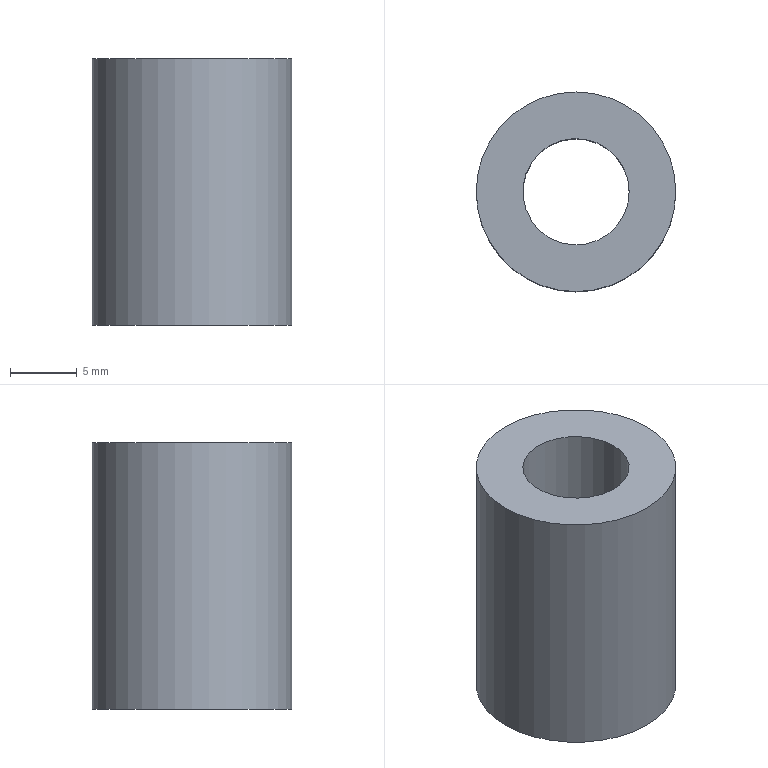Part | NX | features DATUM_CSYS 2, EXTRUDE 1, SKETCH 1 | 1 solid | 4 faces | box 15 x 15 x 20 mm | volume 2529 mm3 | cylinder 2 | plane 2 | commonest cylinder face diameters 8 x1 15 x1
STEP:
#1=CARTESIAN_POINT('',(7.5,0.,20.));
#2=VERTEX_POINT('',#1);
#3=CARTESIAN_POINT('',(0.,0.,20.));
#4=DIRECTION('',(0.,0.,1.));
#5=DIRECTION('',(1.,0.,0.));
#6=AXIS2_PLACEMENT_3D('',#3,#4,#5);
#7=CIRCLE('',#6,7.5);
#8=EDGE_CURVE('',#2,#2,#7,.T.);
#9=ORIENTED_EDGE('',*,*,#8,.F.);
#10=EDGE_LOOP('',(#9));
#11=FACE_BOUND('',#10,.T.);
#12=CARTESIAN_POINT('',(7.5,0.,0.));
#13=VERTEX_POINT('',#12);
#14=CARTESIAN_POINT('',(0.,0.,0.));
#15=DIRECTION('',(0.,0.,1.));
#16=DIRECTION('',(1.,0.,0.));
#17=AXIS2_PLACEMENT_3D('',#14,#15,#16);
#18=CIRCLE('',#17,7.5);
#19=EDGE_CURVE('',#13,#13,#18,.T.);
#20=ORIENTED_EDGE('',*,*,#19,.T.);
#21=EDGE_LOOP('',(#20));
#22=FACE_BOUND('',#21,.T.);
#23=CARTESIAN_POINT('',(0.,0.,20.));
#24=DIRECTION('',(0.,0.,-1.));
#25=DIRECTION('',(-1.,0.,0.));
#26=AXIS2_PLACEMENT_3D('',#23,#24,#25);
#27=CYLINDRICAL_SURFACE('',#26,7.5);
#28=ADVANCED_FACE('',(#11,#22),#27,.T.);
#29=CARTESIAN_POINT('',(4.,0.,20.));
#30=VERTEX_POINT('',#29);
#31=CARTESIAN_POINT('',(0.,0.,20.));
#32=DIRECTION('',(0.,0.,1.));
#33=DIRECTION('',(1.,0.,0.));
#34=AXIS2_PLACEMENT_3D('',#31,#32,#33);
#35=CIRCLE('',#34,4.);
#36=EDGE_CURVE('',#30,#30,#35,.T.);
#37=ORIENTED_EDGE('',*,*,#36,.T.);
#38=EDGE_LOOP('',(#37));
#39=FACE_BOUND('',#38,.T.);
#40=CARTESIAN_POINT('',(4.,0.,0.));
#41=VERTEX_POINT('',#40);
#42=CARTESIAN_POINT('',(0.,0.,0.));
#43=DIRECTION('',(0.,0.,1.));
#44=DIRECTION('',(1.,0.,0.));
#45=AXIS2_PLACEMENT_3D('',#42,#43,#44);
#46=CIRCLE('',#45,4.);
#47=EDGE_CURVE('',#41,#41,#46,.T.);
#48=ORIENTED_EDGE('',*,*,#47,.F.);
#49=EDGE_LOOP('',(#48));
#50=FACE_BOUND('',#49,.T.);
#51=CARTESIAN_POINT('',(0.,0.,20.));
#52=DIRECTION('',(0.,0.,-1.));
#53=DIRECTION('',(-1.,0.,0.));
#54=AXIS2_PLACEMENT_3D('',#51,#52,#53);
#55=CYLINDRICAL_SURFACE('',#54,4.);
#56=ADVANCED_FACE('',(#39,#50),#55,.F.);
#57=ORIENTED_EDGE('',*,*,#8,.T.);
#58=EDGE_LOOP('',(#57));
#59=FACE_BOUND('',#58,.T.);
#60=ORIENTED_EDGE('',*,*,#36,.F.);
#61=EDGE_LOOP('',(#60));
#62=FACE_BOUND('',#61,.T.);
#63=CARTESIAN_POINT('',(0.,0.,20.));
#64=DIRECTION('',(0.,0.,1.));
#65=DIRECTION('',(1.,0.,0.));
#66=AXIS2_PLACEMENT_3D('',#63,#64,#65);
#67=PLANE('',#66);
#68=ADVANCED_FACE('',(#59,#62),#67,.T.);
#69=ORIENTED_EDGE('',*,*,#19,.F.);
#70=EDGE_LOOP('',(#69));
#71=FACE_BOUND('',#70,.T.);
#72=ORIENTED_EDGE('',*,*,#47,.T.);
#73=EDGE_LOOP('',(#72));
#74=FACE_BOUND('',#73,.T.);
#75=CARTESIAN_POINT('',(0.,0.,0.));
#76=DIRECTION('',(0.,0.,1.));
#77=DIRECTION('',(1.,0.,0.));
#78=AXIS2_PLACEMENT_3D('',#75,#76,#77);
#79=PLANE('',#78);
#80=ADVANCED_FACE('',(#71,#74),#79,.F.);
#81=CLOSED_SHELL('',(#28,#56,#68,#80));
#82=MANIFOLD_SOLID_BREP('',#81);
#83=(LENGTH_UNIT()NAMED_UNIT(*)SI_UNIT(.MILLI.,.METRE.));
#84=UNCERTAINTY_MEASURE_WITH_UNIT(LENGTH_MEASURE(0.00001),#83,'','');
#85=(NAMED_UNIT(*)PLANE_ANGLE_UNIT()SI_UNIT($,.RADIAN.));
#86=(NAMED_UNIT(*)SI_UNIT($,.STERADIAN.)SOLID_ANGLE_UNIT());
#87=(GEOMETRIC_REPRESENTATION_CONTEXT(3)GLOBAL_UNCERTAINTY_ASSIGNED_CONTEXT((#84))GLOBAL_UNIT_ASSIGNED_CONTEXT((#83,#85,#86))REPRESENTATION_CONTEXT('',''));
#88=ADVANCED_BREP_SHAPE_REPRESENTATION('',(#82),#87);